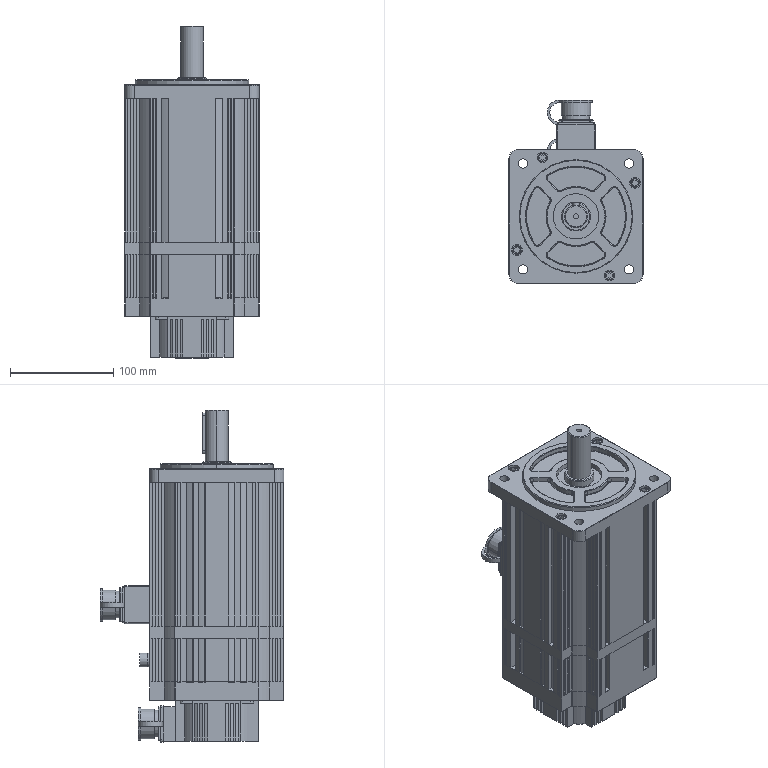Part | SolidWorks | features ICE 34, Fillet 11, MirrorPattern 7, CirPattern 6, Revolution 4, Extrusion 3, PLine 3, Chamfer 2, Sweep 2 | 1 solid | 1616 faces | box 130 x 178 x 321.686 mm | volume 3597344 mm3 | plane 806 | cylinder 596 | torus 192 | sphere 16 | cone 6 | commonest cylinder face diameters 0.4 x332 130 x40 78 x28 6.6 x20 1 x16 2.6 x16